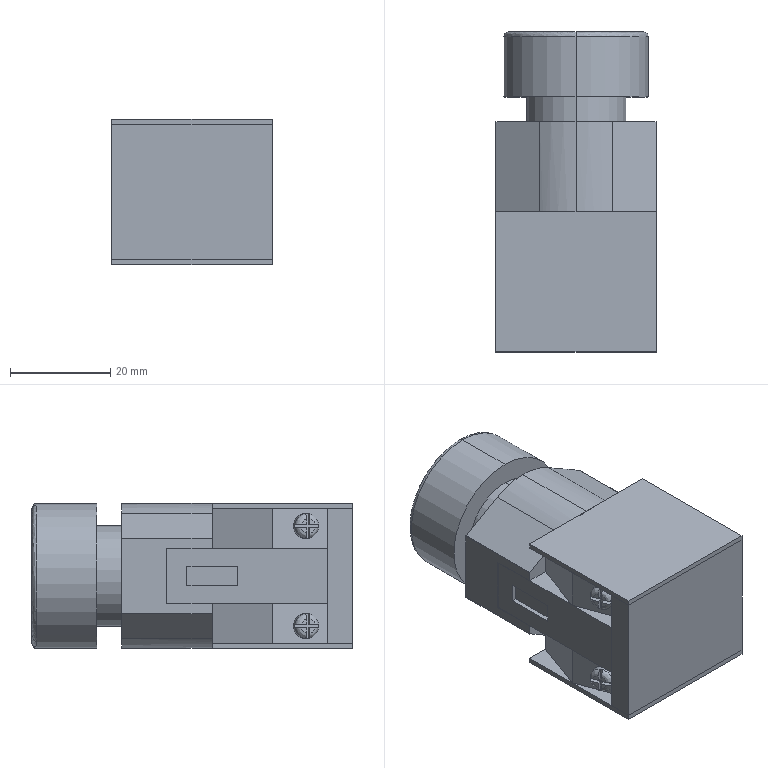Part | SolidWorks | features BaseBody 4 | 4 solids | 211 faces | box 32.2 x 64 x 29 mm | volume 47816 mm3 | plane 174 | cylinder 19 | spline 18 | commonest cylinder face diameters 5 x8 29 x5 20 x2 25.6 x2 26 x2